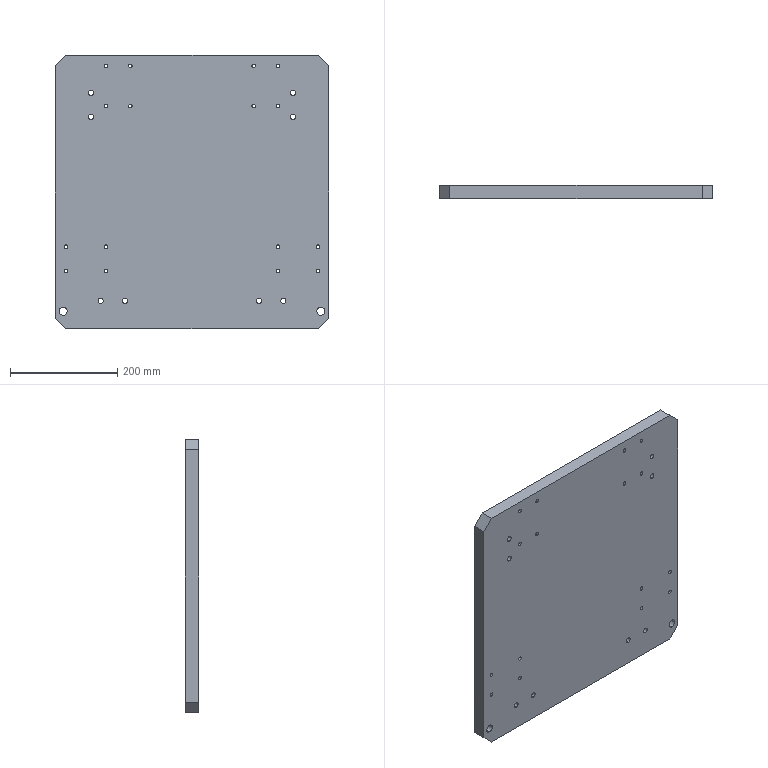Part | SolidWorks | features HoleWzd 4, Chamfer 1, Extrusion 1 | 1 solid | 62 faces | box 510 x 25 x 510 mm | volume 6443430 mm3 | cylinder 52 | plane 10 | commonest cylinder face diameters 6.8 x32 10 x16 15 x4